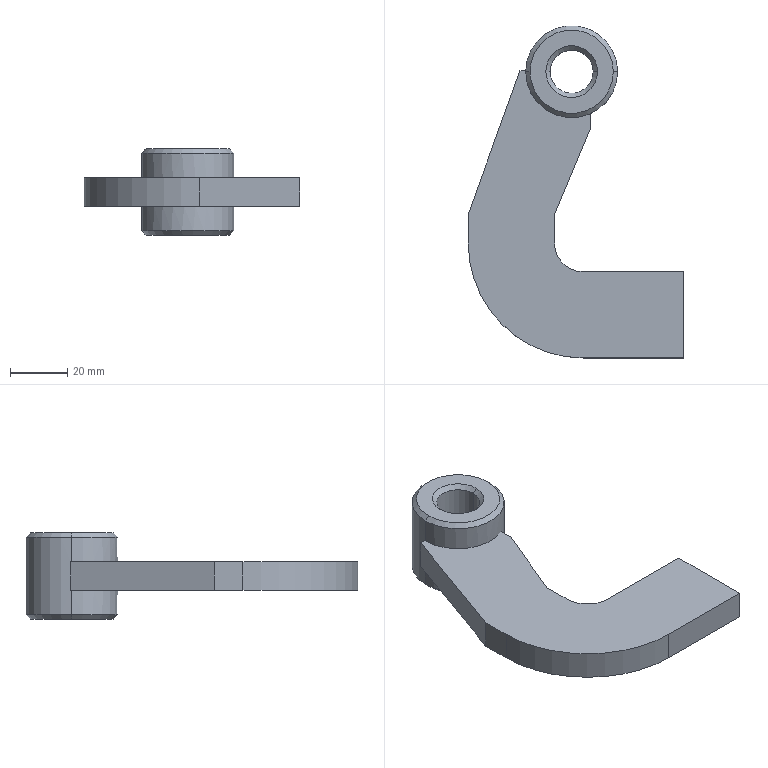Part | STEP file | Input 41 | 1 solid | 27 faces | box 75.005 x 115.604 x 30 mm | volume 55549 mm3 | plane 13 | cone 8 | cylinder 6 | commonest cylinder face diameters 15 x2 32 x2 20 x1 80 x1